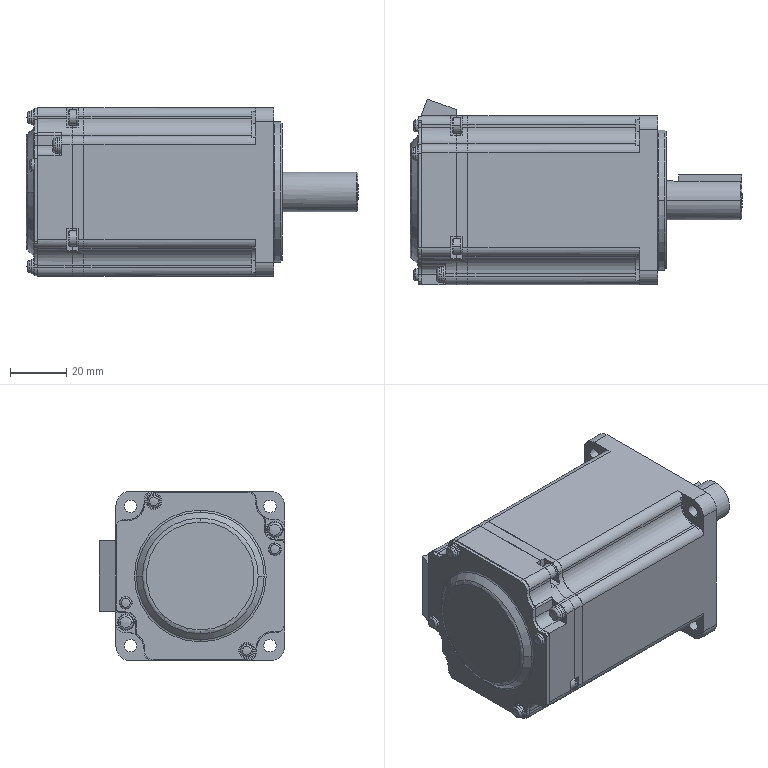Part | SolidWorks | features BaseBody 1 | 1 solid | 358 faces | box 118 x 65.906 x 60 mm | volume 289861 mm3 | plane 165 | cylinder 139 | cone 30 | torus 18 | sphere 6 | commonest cylinder face diameters 6 x40 12 x16 4.5 x8 5.5 x8 5.88 x8 10 x8